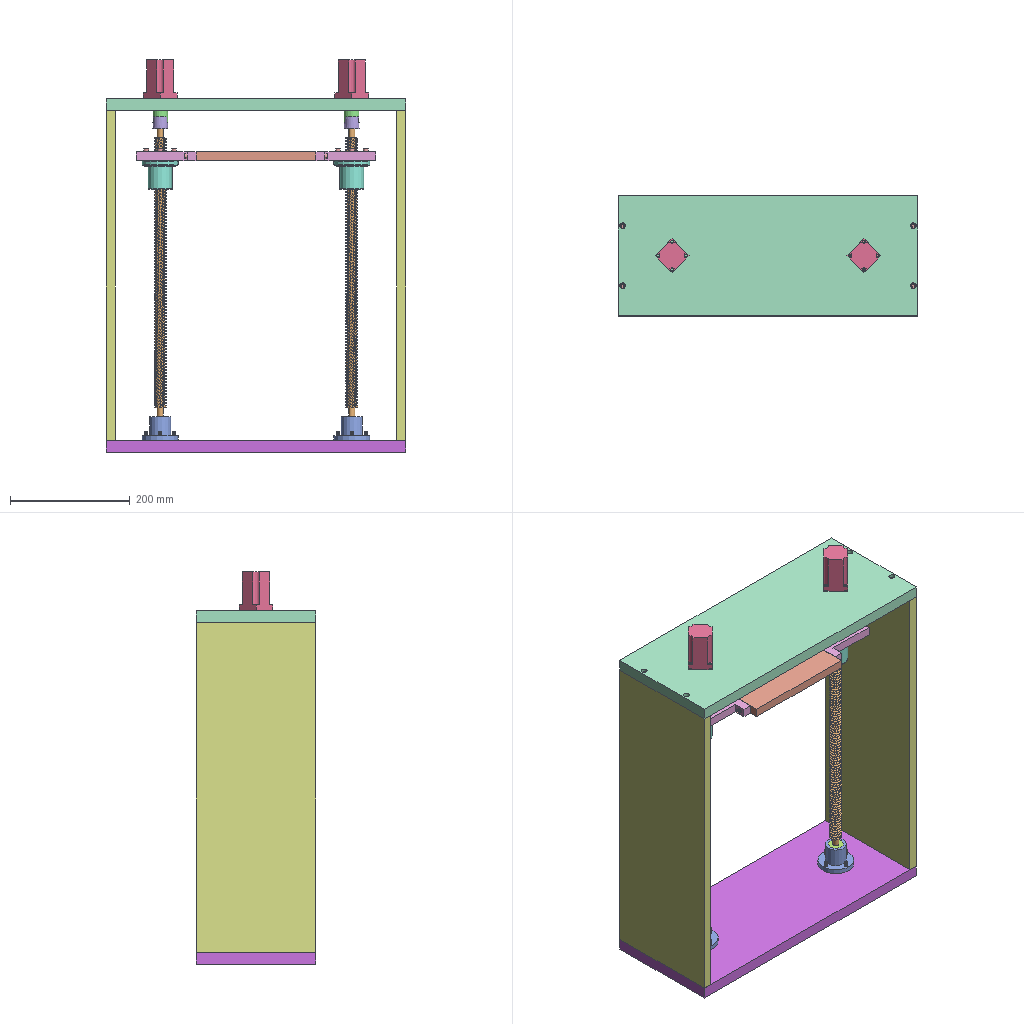Assembly | NX | 12 different items | 46 placed | box 500 x 200 x 655 mm
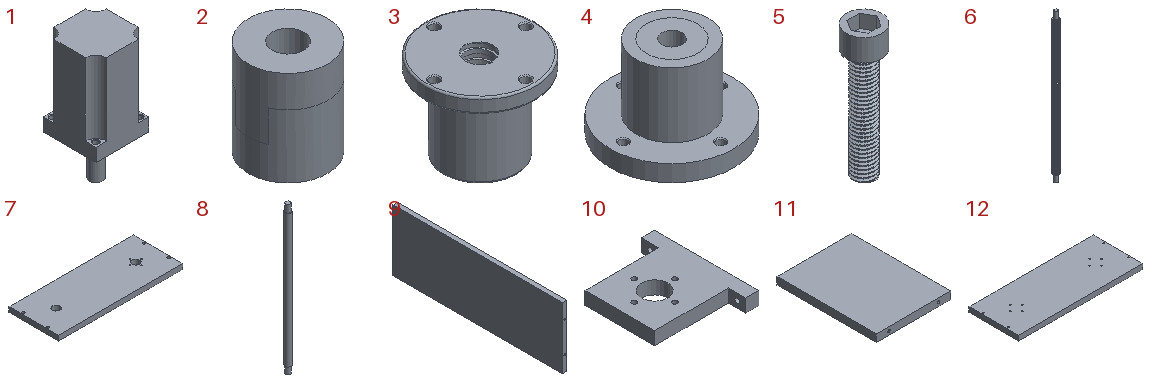Parts list (item | quantity | size | volume | features):
1 | x2 | 40 x 40 x 95 mm | 97876 mm3 | features DATUM_CSYS 5, EXTRUDE 4, SIMPLE HOLE 4, SKETCH 4, SYMBOLIC_THREAD 4, HOLE PACKAGE 1
2 | x2 | 25 x 25 x 30 mm | 12370 mm3 | features EXTRUDE 6, DATUM_CSYS 4, SKETCH 3
3 | x2 | 60 x 60 x 48 mm | 63352 mm3 | features DATUM_CSYS 5, SIMPLE HOLE 4, SKETCH 4, SYMBOLIC_THREAD 4, EXTRUDE 3, BLEND 2, HOLE PACKAGE 1, THREADS 1
4 | x2 | 60 x 60 x 39.6 mm | 47983 mm3 | features DATUM_CSYS 7, SKETCH 6, EXTRUDE 5, SIMPLE HOLE 4, SYMBOLIC_THREAD 4, HOLE PACKAGE 1
5 | x28 | 8 x 8 x 30 mm | 577.822 mm3 | features DATUM_CSYS 4, EXTRUDE 3, SKETCH 3, THREADS 1
6 | x2 | 20 x 20 x 500 mm | 99158 mm3 | features DATUM_CSYS 6, EXTRUDE 5, SKETCH 5, DATUM_PLANE 3, THREADS 1
7 | x1 | 500 x 200 x 20 mm | 1965834 mm3 | features DATUM_CSYS 5, CBORE_HOLE 4, SKETCH 4, EXTRUDE 3, HOLE PACKAGE 1
8 | x1 | 20 x 20 x 500 mm | 150207 mm3 | features DATUM_CSYS 4, EXTRUDE 3, SKETCH 3
9 | x2 | 15 x 550 x 200 mm | 1648864 mm3 | features DATUM_CSYS 4, SIMPLE HOLE 4, SYMBOLIC_THREAD 4, SKETCH 3, EXTRACT_FACE 2, HOLE PACKAGE 2, EXTRUDE 1, Instance Feature 1, Mirror Feature 1
10 | x2 | 100 x 120 x 15 mm | 116259 mm3 | features DATUM_CSYS 3, SIMPLE HOLE 2, SKETCH 2, EXTRUDE 1, HOLE PACKAGE 1
11 | x1 | 150 x 200 x 15 mm | 448864 mm3 | features DATUM_CSYS 4, SIMPLE HOLE 4, SYMBOLIC_THREAD 4, SKETCH 3, EXTRACT_FACE 2, HOLE PACKAGE 2, EXTRUDE 1, Instance Feature 1, Mirror Feature 1
12 | x1 | 500 x 200 x 20 mm | 1988027 mm3 | features CBORE_HOLE 12, DATUM_CSYS 4, SKETCH 3, HOLE PACKAGE 2, EXTRUDE 1
Mates (type | each side: item.copy, entity, surface, feature):
Concentric | 9.1 edge | 7.1 edge | 2 times
Concentric | 12.1 edge | 9.1 edge
Concentric | 1.1 edge | 7.1 edge
Concentric | 11.1 edge | 10.1 edge
Concentric | 4.1 edge | 6.1 edge
Concentric | 4.1 edge | 12.1 edge